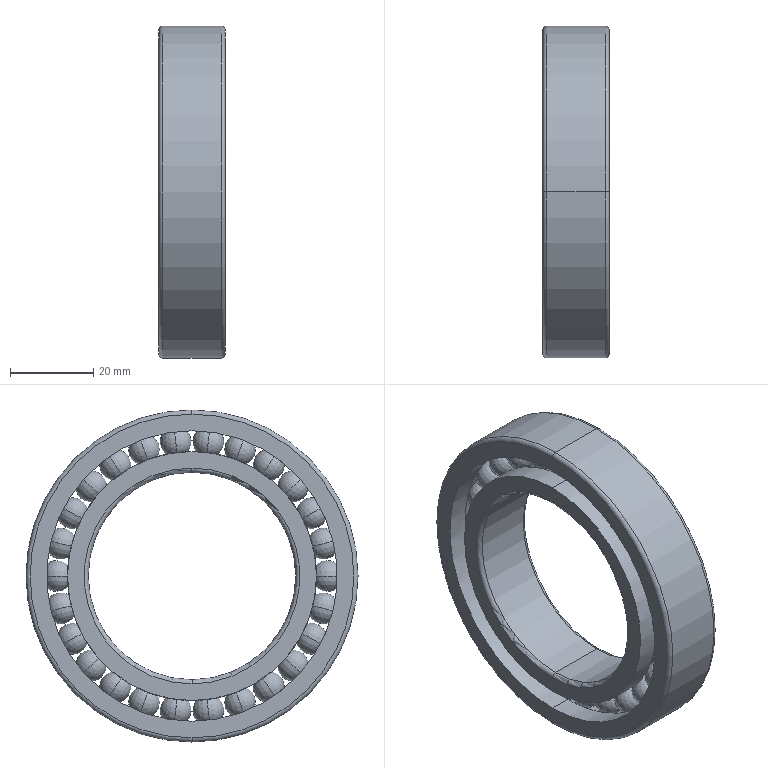Part | STEP file | deep groove ball bearings gb1._Rolling bearings 6010 GB 276-94 | 1 solid | 157 faces | box 16 x 80 x 80 mm | volume 36288 mm3 | torus 89 | sphere 52 | cylinder 12 | plane 4 | commonest cylinder face diameters 60 x4 70 x4 50 x2 80 x2